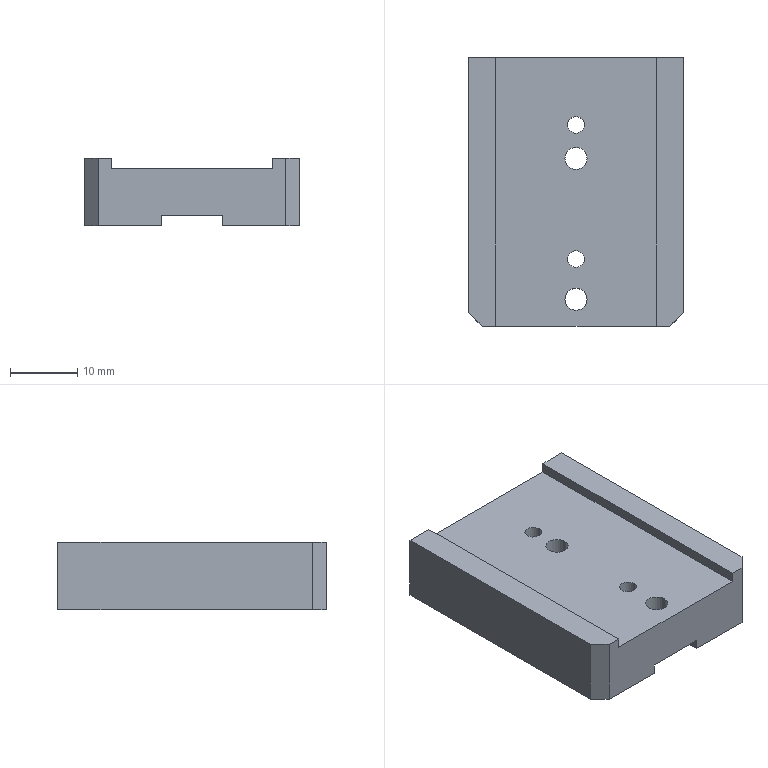Part | STEP file | 11-FG-E00911 | 1 solid | 32 faces | box 32 x 40 x 10 mm | volume 10413 mm3 | plane 16 | cylinder 12 | cone 4 | commonest cylinder face diameters 3.3 x8 2.5 x4
STEP:
#1=CARTESIAN_POINT('',(-24.467,23.184,2.85));
#2=VERTEX_POINT('',#1);
#3=CARTESIAN_POINT('',(-24.467,23.184,6.15));
#4=VERTEX_POINT('',#3);
#5=CARTESIAN_POINT('',(-24.467,23.184,4.5));
#6=DIRECTION('',(0.,1.,0.));
#7=DIRECTION('',(0.,0.,1.));
#8=AXIS2_PLACEMENT_3D('',#5,#6,#7);
#9=CIRCLE('',#8,1.65);
#10=EDGE_CURVE('',#2,#4,#9,.T.);
#11=ORIENTED_EDGE('',*,*,#10,.F.);
#12=CARTESIAN_POINT('',(-24.467,33.284,2.85));
#13=VERTEX_POINT('',#12);
#14=CARTESIAN_POINT('',(-24.467,33.284,2.85));
#15=DIRECTION('',(0.,1.,0.));
#16=VECTOR('',#15,1000.);
#17=LINE('',#14,#16);
#18=EDGE_CURVE('',#2,#13,#17,.T.);
#19=ORIENTED_EDGE('',*,*,#18,.T.);
#20=CARTESIAN_POINT('',(-24.467,33.284,6.15));
#21=VERTEX_POINT('',#20);
#22=CARTESIAN_POINT('',(-24.467,33.284,4.5));
#23=DIRECTION('',(0.,1.,0.));
#24=DIRECTION('',(0.,0.,1.));
#25=AXIS2_PLACEMENT_3D('',#22,#23,#24);
#26=CIRCLE('',#25,1.65);
#27=EDGE_CURVE('',#13,#21,#26,.T.);
#28=ORIENTED_EDGE('',*,*,#27,.T.);
#29=CARTESIAN_POINT('',(-24.467,33.284,6.15));
#30=DIRECTION('',(0.,1.,0.));
#31=VECTOR('',#30,1000.);
#32=LINE('',#29,#31);
#33=EDGE_CURVE('',#4,#21,#32,.T.);
#34=ORIENTED_EDGE('',*,*,#33,.F.);
#35=EDGE_LOOP('',(#11,#19,#28,#34));
#36=FACE_OUTER_BOUND('',#35,.T.);
#37=CARTESIAN_POINT('',(-24.467,33.284,4.5));
#38=DIRECTION('',(0.,1.,0.));
#39=DIRECTION('',(0.,0.,1.));
#40=AXIS2_PLACEMENT_3D('',#37,#38,#39);
#41=CYLINDRICAL_SURFACE('',#40,1.65);
#42=ADVANCED_FACE('',(#36),#41,.F.);
#43=CARTESIAN_POINT('',(-24.467,22.193,4.5));
#44=VERTEX_POINT('',#43);
#45=CARTESIAN_POINT('',(-24.467,23.184,6.15));
#46=DIRECTION('',(0.,0.515,0.8572));
#47=VECTOR('',#46,1000.);
#48=LINE('',#45,#47);
#49=EDGE_CURVE('',#44,#4,#48,.T.);
#50=ORIENTED_EDGE('',*,*,#49,.F.);
#51=CARTESIAN_POINT('',(-24.467,23.184,2.85));
#52=DIRECTION('',(0.,0.515,-0.8572));
#53=VECTOR('',#52,1000.);
#54=LINE('',#51,#53);
#55=EDGE_CURVE('',#44,#2,#54,.T.);
#56=ORIENTED_EDGE('',*,*,#55,.T.);
#57=ORIENTED_EDGE('',*,*,#10,.T.);
#58=EDGE_LOOP('',(#50,#56,#57));
#59=FACE_OUTER_BOUND('',#58,.T.);
#60=CARTESIAN_POINT('',(-24.467,23.184,4.5));
#61=DIRECTION('',(0.,1.,0.));
#62=DIRECTION('',(0.,0.,1.));
#63=AXIS2_PLACEMENT_3D('',#60,#61,#62);
#64=CONICAL_SURFACE('',#63,1.65,1.03);
#65=ADVANCED_FACE('',(#59),#64,.F.);
#66=CARTESIAN_POINT('',(-9.467,23.184,2.85));
#67=VERTEX_POINT('',#66);
#68=CARTESIAN_POINT('',(-9.467,23.184,6.15));
#69=VERTEX_POINT('',#68);
#70=CARTESIAN_POINT('',(-9.467,23.184,4.5));
#71=DIRECTION('',(0.,1.,0.));
#72=DIRECTION('',(0.,0.,1.));
#73=AXIS2_PLACEMENT_3D('',#70,#71,#72);
#74=CIRCLE('',#73,1.65);
#75=EDGE_CURVE('',#67,#69,#74,.T.);
#76=ORIENTED_EDGE('',*,*,#75,.F.);
#77=CARTESIAN_POINT('',(-9.467,33.284,2.85));
#78=VERTEX_POINT('',#77);
#79=CARTESIAN_POINT('',(-9.467,33.284,2.85));
#80=DIRECTION('',(0.,1.,0.));
#81=VECTOR('',#80,1000.);
#82=LINE('',#79,#81);
#83=EDGE_CURVE('',#67,#78,#82,.T.);
#84=ORIENTED_EDGE('',*,*,#83,.T.);
#85=CARTESIAN_POINT('',(-9.467,33.284,6.15));
#86=VERTEX_POINT('',#85);
#87=CARTESIAN_POINT('',(-9.467,33.284,4.5));
#88=DIRECTION('',(0.,1.,0.));
#89=DIRECTION('',(0.,0.,1.));
#90=AXIS2_PLACEMENT_3D('',#87,#88,#89);
#91=CIRCLE('',#90,1.65);
#92=EDGE_CURVE('',#78,#86,#91,.T.);
#93=ORIENTED_EDGE('',*,*,#92,.T.);
#94=CARTESIAN_POINT('',(-9.467,33.284,6.15));
#95=DIRECTION('',(0.,1.,0.));
#96=VECTOR('',#95,1000.);
#97=LINE('',#94,#96);
#98=EDGE_CURVE('',#69,#86,#97,.T.);
#99=ORIENTED_EDGE('',*,*,#98,.F.);
#100=EDGE_LOOP('',(#76,#84,#93,#99));
#101=FACE_OUTER_BOUND('',#100,.T.);
#102=CARTESIAN_POINT('',(-9.467,33.284,4.5));
#103=DIRECTION('',(0.,1.,0.));
#104=DIRECTION('',(0.,0.,1.));
#105=AXIS2_PLACEMENT_3D('',#102,#103,#104);
#106=CYLINDRICAL_SURFACE('',#105,1.65);
#107=ADVANCED_FACE('',(#101),#106,.F.);
#108=CARTESIAN_POINT('',(-9.467,22.193,4.5));
#109=VERTEX_POINT('',#108);
#110=CARTESIAN_POINT('',(-9.467,23.184,6.15));
#111=DIRECTION('',(0.,0.515,0.8572));
#112=VECTOR('',#111,1000.);
#113=LINE('',#110,#112);
#114=EDGE_CURVE('',#109,#69,#113,.T.);
#115=ORIENTED_EDGE('',*,*,#114,.F.);
#116=CARTESIAN_POINT('',(-9.467,23.184,2.85));
#117=DIRECTION('',(0.,0.515,-0.8572));
#118=VECTOR('',#117,1000.);
#119=LINE('',#116,#118);
#120=EDGE_CURVE('',#109,#67,#119,.T.);
#121=ORIENTED_EDGE('',*,*,#120,.T.);
#122=ORIENTED_EDGE('',*,*,#75,.T.);
#123=EDGE_LOOP('',(#115,#121,#122));
#124=FACE_OUTER_BOUND('',#123,.T.);
#125=CARTESIAN_POINT('',(-9.467,23.184,4.5));
#126=DIRECTION('',(0.,1.,0.));
#127=DIRECTION('',(0.,0.,1.));
#128=AXIS2_PLACEMENT_3D('',#125,#126,#127);
#129=CONICAL_SURFACE('',#128,1.65,1.03);
#130=ADVANCED_FACE('',(#124),#129,.F.);
#131=CARTESIAN_POINT('',(-18.617,-2.716,1.5));
#132=VERTEX_POINT('',#131);
#133=CARTESIAN_POINT('',(-15.317,-2.716,1.5));
#134=VERTEX_POINT('',#133);
#135=CARTESIAN_POINT('',(-16.967,-2.716,1.5));
#136=DIRECTION('',(0.,0.,1.));
#137=DIRECTION('',(1.,0.,0.));
#138=AXIS2_PLACEMENT_3D('',#135,#136,#137);
#139=CIRCLE('',#138,1.65);
#140=EDGE_CURVE('',#132,#134,#139,.T.);
#141=ORIENTED_EDGE('',*,*,#140,.F.);
#142=CARTESIAN_POINT('',(-18.617,-2.716,8.5));
#143=VERTEX_POINT('',#142);
#144=CARTESIAN_POINT('',(-18.617,-2.716,8.5));
#145=DIRECTION('',(0.,0.,1.));
#146=VECTOR('',#145,1000.);
#147=LINE('',#144,#146);
#148=EDGE_CURVE('',#132,#143,#147,.T.);
#149=ORIENTED_EDGE('',*,*,#148,.T.);
#150=CARTESIAN_POINT('',(-15.317,-2.716,8.5));
#151=VERTEX_POINT('',#150);
#152=CARTESIAN_POINT('',(-16.967,-2.716,8.5));
#153=DIRECTION('',(0.,0.,1.));
#154=DIRECTION('',(1.,0.,0.));
#155=AXIS2_PLACEMENT_3D('',#152,#153,#154);
#156=CIRCLE('',#155,1.65);
#157=EDGE_CURVE('',#143,#151,#156,.T.);
#158=ORIENTED_EDGE('',*,*,#157,.T.);
#159=CARTESIAN_POINT('',(-15.317,-2.716,8.5));
#160=DIRECTION('',(0.,0.,1.));
#161=VECTOR('',#160,1000.);
#162=LINE('',#159,#161);
#163=EDGE_CURVE('',#134,#151,#162,.T.);
#164=ORIENTED_EDGE('',*,*,#163,.F.);
#165=EDGE_LOOP('',(#141,#149,#158,#164));
#166=FACE_OUTER_BOUND('',#165,.T.);
#167=CARTESIAN_POINT('',(-16.967,-2.716,8.5));
#168=DIRECTION('',(0.,0.,1.));
#169=DIRECTION('',(1.,0.,0.));
#170=AXIS2_PLACEMENT_3D('',#167,#168,#169);
#171=CYLINDRICAL_SURFACE('',#170,1.65);
#172=ADVANCED_FACE('',(#166),#171,.F.);
#173=CARTESIAN_POINT('',(-18.617,18.284,1.5));
#174=VERTEX_POINT('',#173);
#175=CARTESIAN_POINT('',(-15.317,18.284,1.5));
#176=VERTEX_POINT('',#175);
#177=CARTESIAN_POINT('',(-16.967,18.284,1.5));
#178=DIRECTION('',(0.,0.,1.));
#179=DIRECTION('',(1.,0.,0.));
#180=AXIS2_PLACEMENT_3D('',#177,#178,#179);
#181=CIRCLE('',#180,1.65);
#182=EDGE_CURVE('',#174,#176,#181,.T.);
#183=ORIENTED_EDGE('',*,*,#182,.F.);
#184=CARTESIAN_POINT('',(-18.617,18.284,8.5));
#185=VERTEX_POINT('',#184);
#186=CARTESIAN_POINT('',(-18.617,18.284,8.5));
#187=DIRECTION('',(0.,0.,1.));
#188=VECTOR('',#187,1000.);
#189=LINE('',#186,#188);
#190=EDGE_CURVE('',#174,#185,#189,.T.);
#191=ORIENTED_EDGE('',*,*,#190,.T.);
#192=CARTESIAN_POINT('',(-15.317,18.284,8.5));
#193=VERTEX_POINT('',#192);
#194=CARTESIAN_POINT('',(-16.967,18.284,8.5));
#195=DIRECTION('',(0.,0.,1.));
#196=DIRECTION('',(1.,0.,0.));
#197=AXIS2_PLACEMENT_3D('',#194,#195,#196);
#198=CIRCLE('',#197,1.65);
#199=EDGE_CURVE('',#185,#193,#198,.T.);
#200=ORIENTED_EDGE('',*,*,#199,.T.);
#201=CARTESIAN_POINT('',(-15.317,18.284,8.5));
#202=DIRECTION('',(0.,0.,1.));
#203=VECTOR('',#202,1000.);
#204=LINE('',#201,#203);
#205=EDGE_CURVE('',#176,#193,#204,.T.);
#206=ORIENTED_EDGE('',*,*,#205,.F.);
#207=EDGE_LOOP('',(#183,#191,#200,#206));
#208=FACE_OUTER_BOUND('',#207,.T.);
#209=CARTESIAN_POINT('',(-16.967,18.284,8.5));
#210=DIRECTION('',(0.,0.,1.));
#211=DIRECTION('',(1.,0.,0.));
#212=AXIS2_PLACEMENT_3D('',#209,#210,#211);
#213=CYLINDRICAL_SURFACE('',#212,1.65);
#214=ADVANCED_FACE('',(#208),#213,.F.);
#215=CARTESIAN_POINT('',(-18.217,3.284,8.5));
#216=VERTEX_POINT('',#215);
#217=CARTESIAN_POINT('',(-15.717,3.284,8.5));
#218=VERTEX_POINT('',#217);
#219=CARTESIAN_POINT('',(-16.967,3.284,8.5));
#220=DIRECTION('',(0.,0.,1.));
#221=DIRECTION('',(1.,0.,0.));
#222=AXIS2_PLACEMENT_3D('',#219,#220,#221);
#223=CIRCLE('',#222,1.25);
#224=EDGE_CURVE('',#216,#218,#223,.T.);
#225=ORIENTED_EDGE('',*,*,#224,.T.);
#226=CARTESIAN_POINT('',(-15.717,3.284,1.5));
#227=VERTEX_POINT('',#226);
#228=CARTESIAN_POINT('',(-15.717,3.284,1.5));
#229=DIRECTION('',(0.,0.,-1.));
#230=VECTOR('',#229,1000.);
#231=LINE('',#228,#230);
#232=EDGE_CURVE('',#218,#227,#231,.T.);
#233=ORIENTED_EDGE('',*,*,#232,.T.);
#234=CARTESIAN_POINT('',(-18.217,3.284,1.5));
#235=VERTEX_POINT('',#234);
#236=CARTESIAN_POINT('',(-16.967,3.284,1.5));
#237=DIRECTION('',(0.,0.,-1.));
#238=DIRECTION('',(-1.,0.,0.));
#239=AXIS2_PLACEMENT_3D('',#236,#237,#238);
#240=CIRCLE('',#239,1.25);
#241=EDGE_CURVE('',#227,#235,#240,.T.);
#242=ORIENTED_EDGE('',*,*,#241,.T.);
#243=CARTESIAN_POINT('',(-18.217,3.284,1.5));
#244=DIRECTION('',(0.,0.,-1.));
#245=VECTOR('',#244,1000.);
#246=LINE('',#243,#245);
#247=EDGE_CURVE('',#216,#235,#246,.T.);
#248=ORIENTED_EDGE('',*,*,#247,.F.);
#249=EDGE_LOOP('',(#225,#233,#242,#248));
#250=FACE_OUTER_BOUND('',#249,.T.);
#251=CARTESIAN_POINT('',(-16.967,3.284,1.5));
#252=DIRECTION('',(0.,0.,-1.));
#253=DIRECTION('',(-1.,0.,0.));
#254=AXIS2_PLACEMENT_3D('',#251,#252,#253);
#255=CYLINDRICAL_SURFACE('',#254,1.25);
#256=ADVANCED_FACE('',(#250),#255,.F.);
#257=CARTESIAN_POINT('',(-18.217,23.284,8.5));
#258=VERTEX_POINT('',#257);
#259=CARTESIAN_POINT('',(-15.717,23.284,8.5));
#260=VERTEX_POINT('',#259);
#261=CARTESIAN_POINT('',(-16.967,23.284,8.5));
#262=DIRECTION('',(0.,0.,1.));
#263=DIRECTION('',(1.,0.,0.));
#264=AXIS2_PLACEMENT_3D('',#261,#262,#263);
#265=CIRCLE('',#264,1.25);
#266=EDGE_CURVE('',#258,#260,#265,.T.);
#267=ORIENTED_EDGE('',*,*,#266,.T.);
#268=CARTESIAN_POINT('',(-15.717,23.284,1.5));
#269=VERTEX_POINT('',#268);
#270=CARTESIAN_POINT('',(-15.717,23.284,1.5));
#271=DIRECTION('',(0.,0.,-1.));
#272=VECTOR('',#271,1000.);
#273=LINE('',#270,#272);
#274=EDGE_CURVE('',#260,#269,#273,.T.);
#275=ORIENTED_EDGE('',*,*,#274,.T.);
#276=CARTESIAN_POINT('',(-18.217,23.284,1.5));
#277=VERTEX_POINT('',#276);
#278=CARTESIAN_POINT('',(-16.967,23.284,1.5));
#279=DIRECTION('',(0.,0.,-1.));
#280=DIRECTION('',(-1.,0.,0.));
#281=AXIS2_PLACEMENT_3D('',#278,#279,#280);
#282=CIRCLE('',#281,1.25);
#283=EDGE_CURVE('',#269,#277,#282,.T.);
#284=ORIENTED_EDGE('',*,*,#283,.T.);
#285=CARTESIAN_POINT('',(-18.217,23.284,1.5));
#286=DIRECTION('',(0.,0.,-1.));
#287=VECTOR('',#286,1000.);
#288=LINE('',#285,#287);
#289=EDGE_CURVE('',#258,#277,#288,.T.);
#290=ORIENTED_EDGE('',*,*,#289,.F.);
#291=EDGE_LOOP('',(#267,#275,#284,#290));
#292=FACE_OUTER_BOUND('',#291,.T.);
#293=CARTESIAN_POINT('',(-16.967,23.284,1.5));
#294=DIRECTION('',(0.,0.,-1.));
#295=DIRECTION('',(-1.,0.,0.));
#296=AXIS2_PLACEMENT_3D('',#293,#294,#295);
#297=CYLINDRICAL_SURFACE('',#296,1.25);
#298=ADVANCED_FACE('',(#292),#297,.F.);
#299=CARTESIAN_POINT('',(-12.467,-6.716,0.));
#300=VERTEX_POINT('',#299);
#301=CARTESIAN_POINT('',(-2.967,-6.716,0.));
#302=VERTEX_POINT('',#301);
#303=CARTESIAN_POINT('',(-32.967,-6.716,0.));
#304=DIRECTION('',(1.,0.,0.));
#305=VECTOR('',#304,1000.);
#306=LINE('',#303,#305);
#307=EDGE_CURVE('',#300,#302,#306,.T.);
#308=ORIENTED_EDGE('',*,*,#307,.F.);
#309=CARTESIAN_POINT('',(-12.467,33.284,0.));
#310=VERTEX_POINT('',#309);
#311=CARTESIAN_POINT('',(-12.467,-6.716,0.));
#312=DIRECTION('',(0.,1.,0.));
#313=VECTOR('',#312,1000.);
#314=LINE('',#311,#313);
#315=EDGE_CURVE('',#300,#310,#314,.T.);
#316=ORIENTED_EDGE('',*,*,#315,.T.);
#317=CARTESIAN_POINT('',(-0.9669,33.284,0.));
#318=VERTEX_POINT('',#317);
#319=CARTESIAN_POINT('',(-32.967,33.284,0.));
#320=DIRECTION('',(-1.,0.,0.));
#321=VECTOR('',#320,1000.);
#322=LINE('',#319,#321);
#323=EDGE_CURVE('',#318,#310,#322,.T.);
#324=ORIENTED_EDGE('',*,*,#323,.F.);
#325=CARTESIAN_POINT('',(-0.9669,-4.716,0.));
#326=VERTEX_POINT('',#325);
#327=CARTESIAN_POINT('',(-0.9669,33.284,0.));
#328=DIRECTION('',(0.,1.,0.));
#329=VECTOR('',#328,1000.);
#330=LINE('',#327,#329);
#331=EDGE_CURVE('',#326,#318,#330,.T.);
#332=ORIENTED_EDGE('',*,*,#331,.F.);
#333=CARTESIAN_POINT('',(-0.9669,-4.716,0.));
#334=DIRECTION('',(-0.7071,-0.7071,0.));
#335=VECTOR('',#334,1000.);
#336=LINE('',#333,#335);
#337=EDGE_CURVE('',#326,#302,#336,.T.);
#338=ORIENTED_EDGE('',*,*,#337,.T.);
#339=EDGE_LOOP('',(#308,#316,#324,#332,#338));
#340=FACE_OUTER_BOUND('',#339,.T.);
#341=CARTESIAN_POINT('',(-32.967,-6.716,0.));
#342=DIRECTION('',(0.,0.,1.));
#343=DIRECTION('',(1.,0.,0.));
#344=AXIS2_PLACEMENT_3D('',#341,#342,#343);
#345=PLANE('',#344);
#346=ADVANCED_FACE('',(#340),#345,.F.);
#347=CARTESIAN_POINT('',(-24.467,33.284,4.5));
#348=DIRECTION('',(0.,1.,0.));
#349=DIRECTION('',(0.,0.,1.));
#350=AXIS2_PLACEMENT_3D('',#347,#348,#349);
#351=CIRCLE('',#350,1.65);
#352=EDGE_CURVE('',#21,#13,#351,.T.);
#353=ORIENTED_EDGE('',*,*,#352,.F.);
#354=ORIENTED_EDGE('',*,*,#27,.F.);
#355=EDGE_LOOP('',(#353,#354));
#356=FACE_BOUND('',#355,.T.);
#357=CARTESIAN_POINT('',(-9.467,33.284,4.5));
#358=DIRECTION('',(0.,1.,0.));
#359=DIRECTION('',(0.,0.,1.));
#360=AXIS2_PLACEMENT_3D('',#357,#358,#359);
#361=CIRCLE('',#360,1.65);
#362=EDGE_CURVE('',#86,#78,#361,.T.);
#363=ORIENTED_EDGE('',*,*,#362,.F.);
#364=ORIENTED_EDGE('',*,*,#92,.F.);
#365=EDGE_LOOP('',(#363,#364));
#366=FACE_BOUND('',#365,.T.);
#367=ORIENTED_EDGE('',*,*,#323,.T.);
#368=CARTESIAN_POINT('',(-12.467,33.284,1.5));
#369=VERTEX_POINT('',#368);
#370=CARTESIAN_POINT('',(-12.467,33.284,10.));
#371=DIRECTION('',(0.,0.,1.));
#372=VECTOR('',#371,1000.);
#373=LINE('',#370,#372);
#374=EDGE_CURVE('',#310,#369,#373,.T.);
#375=ORIENTED_EDGE('',*,*,#374,.T.);
#376=CARTESIAN_POINT('',(-21.467,33.284,1.5));
#377=VERTEX_POINT('',#376);
#378=CARTESIAN_POINT('',(-32.967,33.284,1.5));
#379=DIRECTION('',(-1.,0.,0.));
#380=VECTOR('',#379,1000.);
#381=LINE('',#378,#380);
#382=EDGE_CURVE('',#369,#377,#381,.T.);
#383=ORIENTED_EDGE('',*,*,#382,.T.);
#384=CARTESIAN_POINT('',(-21.467,33.284,0.));
#385=VERTEX_POINT('',#384);
#386=CARTESIAN_POINT('',(-21.467,33.284,10.));
#387=DIRECTION('',(0.,0.,-1.));
#388=VECTOR('',#387,1000.);
#389=LINE('',#386,#388);
#390=EDGE_CURVE('',#377,#385,#389,.T.);
#391=ORIENTED_EDGE('',*,*,#390,.T.);
#392=CARTESIAN_POINT('',(-32.967,33.284,0.));
#393=VERTEX_POINT('',#392);
#394=CARTESIAN_POINT('',(-32.967,33.284,0.));
#395=DIRECTION('',(-1.,0.,0.));
#396=VECTOR('',#395,1000.);
#397=LINE('',#394,#396);
#398=EDGE_CURVE('',#385,#393,#397,.T.);
#399=ORIENTED_EDGE('',*,*,#398,.T.);
#400=CARTESIAN_POINT('',(-32.967,33.284,10.));
#401=VERTEX_POINT('',#400);
#402=CARTESIAN_POINT('',(-32.967,33.284,10.));
#403=DIRECTION('',(0.,0.,-1.));
#404=VECTOR('',#403,1000.);
#405=LINE('',#402,#404);
#406=EDGE_CURVE('',#401,#393,#405,.T.);
#407=ORIENTED_EDGE('',*,*,#406,.F.);
#408=CARTESIAN_POINT('',(-28.967,33.284,10.));
#409=VERTEX_POINT('',#408);
#410=CARTESIAN_POINT('',(-32.967,33.284,10.));
#411=DIRECTION('',(-1.,0.,0.));
#412=VECTOR('',#411,1000.);
#413=LINE('',#410,#412);
#414=EDGE_CURVE('',#409,#401,#413,.T.);
#415=ORIENTED_EDGE('',*,*,#414,.F.);
#416=CARTESIAN_POINT('',(-28.967,33.284,8.5));
#417=VERTEX_POINT('',#416);
#418=CARTESIAN_POINT('',(-28.967,33.284,8.5));
#419=DIRECTION('',(0.,0.,1.));
#420=VECTOR('',#419,1000.);
#421=LINE('',#418,#420);
#422=EDGE_CURVE('',#417,#409,#421,.T.);
#423=ORIENTED_EDGE('',*,*,#422,.F.);
#424=CARTESIAN_POINT('',(-4.967,33.284,8.5));
#425=VERTEX_POINT('',#424);
#426=CARTESIAN_POINT('',(-28.967,33.284,8.5));
#427=DIRECTION('',(-1.,0.,0.));
#428=VECTOR('',#427,1000.);
#429=LINE('',#426,#428);
#430=EDGE_CURVE('',#425,#417,#429,.T.);
#431=ORIENTED_EDGE('',*,*,#430,.F.);
#432=CARTESIAN_POINT('',(-4.967,33.284,10.));
#433=VERTEX_POINT('',#432);
#434=CARTESIAN_POINT('',(-4.967,33.284,8.5));
#435=DIRECTION('',(0.,0.,1.));
#436=VECTOR('',#435,1000.);
#437=LINE('',#434,#436);
#438=EDGE_CURVE('',#425,#433,#437,.T.);
#439=ORIENTED_EDGE('',*,*,#438,.T.);
#440=CARTESIAN_POINT('',(-0.9669,33.284,10.));
#441=VERTEX_POINT('',#440);
#442=CARTESIAN_POINT('',(-32.967,33.284,10.));
#443=DIRECTION('',(-1.,0.,0.));
#444=VECTOR('',#443,1000.);
#445=LINE('',#442,#444);
#446=EDGE_CURVE('',#441,#433,#445,.T.);
#447=ORIENTED_EDGE('',*,*,#446,.F.);
#448=CARTESIAN_POINT('',(-0.9669,33.284,10.));
#449=DIRECTION('',(0.,0.,-1.));
#450=VECTOR('',#449,1000.);
#451=LINE('',#448,#450);
#452=EDGE_CURVE('',#441,#318,#451,.T.);
#453=ORIENTED_EDGE('',*,*,#452,.T.);
#454=EDGE_LOOP('',(#367,#375,#383,#391,#399,#407,#415,#423,#431,#439,#447,#453));
#455=FACE_OUTER_BOUND('',#454,.T.);
#456=CARTESIAN_POINT('',(-32.967,33.284,10.));
#457=DIRECTION('',(0.,-1.,0.));
#458=DIRECTION('',(0.,0.,-1.));
#459=AXIS2_PLACEMENT_3D('',#456,#457,#458);
#460=PLANE('',#459);
#461=ADVANCED_FACE('',(#356,#366,#455),#460,.F.);
#462=CARTESIAN_POINT('',(-32.967,-4.716,10.));
#463=VERTEX_POINT('',#462);
#464=CARTESIAN_POINT('',(-32.967,33.284,10.));
#465=DIRECTION('',(0.,-1.,0.));
#466=VECTOR('',#465,1000.);
#467=LINE('',#464,#466);
#468=EDGE_CURVE('',#401,#463,#467,.T.);
#469=ORIENTED_EDGE('',*,*,#468,.T.);
#470=CARTESIAN_POINT('',(-30.967,-6.716,10.));
#471=VERTEX_POINT('',#470);
#472=CARTESIAN_POINT('',(-31.967,-5.716,10.));
#473=DIRECTION('',(0.7071,-0.7071,0.));
#474=VECTOR('',#473,1000.);
#475=LINE('',#472,#474);
#476=EDGE_CURVE('',#463,#471,#475,.T.);
#477=ORIENTED_EDGE('',*,*,#476,.T.);
#478=CARTESIAN_POINT('',(-28.967,-6.716,10.));
#479=VERTEX_POINT('',#478);
#480=CARTESIAN_POINT('',(-32.967,-6.716,10.));
#481=DIRECTION('',(1.,0.,0.));
#482=VECTOR('',#481,1000.);
#483=LINE('',#480,#482);
#484=EDGE_CURVE('',#471,#479,#483,.T.);
#485=ORIENTED_EDGE('',*,*,#484,.T.);
#486=CARTESIAN_POINT('',(-28.967,33.284,10.));
#487=DIRECTION('',(0.,-1.,0.));
#488=VECTOR('',#487,1000.);
#489=LINE('',#486,#488);
#490=EDGE_CURVE('',#409,#479,#489,.T.);
#491=ORIENTED_EDGE('',*,*,#490,.F.);
#492=ORIENTED_EDGE('',*,*,#414,.T.);
#493=EDGE_LOOP('',(#469,#477,#485,#491,#492));
#494=FACE_OUTER_BOUND('',#493,.T.);
#495=CARTESIAN_POINT('',(-32.967,-6.716,10.));
#496=DIRECTION('',(0.,0.,1.));
#497=DIRECTION('',(1.,0.,0.));
#498=AXIS2_PLACEMENT_3D('',#495,#496,#497);
#499=PLANE('',#498);
#500=ADVANCED_FACE('',(#494),#499,.T.);
#501=CARTESIAN_POINT('',(-32.967,-4.716,0.));
#502=VERTEX_POINT('',#501);
#503=CARTESIAN_POINT('',(-32.967,33.284,0.));
#504=DIRECTION('',(0.,-1.,0.));
#505=VECTOR('',#504,1000.);
#506=LINE('',#503,#505);
#507=EDGE_CURVE('',#393,#502,#506,.T.);
#508=ORIENTED_EDGE('',*,*,#507,.T.);
#509=CARTESIAN_POINT('',(-32.967,-4.716,10.));
#510=DIRECTION('',(0.,0.,1.));
#511=VECTOR('',#510,1000.);
#512=LINE('',#509,#511);
#513=EDGE_CURVE('',#502,#463,#512,.T.);
#514=ORIENTED_EDGE('',*,*,#513,.T.);
#515=ORIENTED_EDGE('',*,*,#468,.F.);
#516=ORIENTED_EDGE('',*,*,#406,.T.);
#517=EDGE_LOOP('',(#508,#514,#515,#516));
#518=FACE_OUTER_BOUND('',#517,.T.);
#519=CARTESIAN_POINT('',(-32.967,33.284,10.));
#520=DIRECTION('',(1.,0.,0.));
#521=DIRECTION('',(0.,1.,0.));
#522=AXIS2_PLACEMENT_3D('',#519,#520,#521);
#523=PLANE('',#522);
#524=ADVANCED_FACE('',(#518),#523,.F.);
#525=CARTESIAN_POINT('',(-12.467,-6.716,1.5));
#526=VERTEX_POINT('',#525);
#527=CARTESIAN_POINT('',(-21.467,-6.716,1.5));
#528=VERTEX_POINT('',#527);
#529=CARTESIAN_POINT('',(-12.467,-6.716,1.5));
#530=DIRECTION('',(-1.,0.,0.));
#531=VECTOR('',#530,1000.);
#532=LINE('',#529,#531);
#533=EDGE_CURVE('',#526,#528,#532,.T.);
#534=ORIENTED_EDGE('',*,*,#533,.F.);
#535=CARTESIAN_POINT('',(-12.467,-6.716,0.));
#536=DIRECTION('',(0.,0.,1.));
#537=VECTOR('',#536,1000.);
#538=LINE('',#535,#537);
#539=EDGE_CURVE('',#300,#526,#538,.T.);
#540=ORIENTED_EDGE('',*,*,#539,.F.);
#541=ORIENTED_EDGE('',*,*,#307,.T.);
#542=CARTESIAN_POINT('',(-2.967,-6.716,10.));
#543=VERTEX_POINT('',#542);
#544=CARTESIAN_POINT('',(-2.967,-6.716,10.));
#545=DIRECTION('',(0.,0.,1.));
#546=VECTOR('',#545,1000.);
#547=LINE('',#544,#546);
#548=EDGE_CURVE('',#302,#543,#547,.T.);
#549=ORIENTED_EDGE('',*,*,#548,.T.);
#550=CARTESIAN_POINT('',(-4.967,-6.716,10.));
#551=VERTEX_POINT('',#550);
#552=CARTESIAN_POINT('',(-32.967,-6.716,10.));
#553=DIRECTION('',(1.,0.,0.));
#554=VECTOR('',#553,1000.);
#555=LINE('',#552,#554);
#556=EDGE_CURVE('',#551,#543,#555,.T.);
#557=ORIENTED_EDGE('',*,*,#556,.F.);
#558=CARTESIAN_POINT('',(-4.967,-6.716,8.5));
#559=VERTEX_POINT('',#558);
#560=CARTESIAN_POINT('',(-4.967,-6.716,8.5));
#561=DIRECTION('',(0.,0.,1.));
#562=VECTOR('',#561,1000.);
#563=LINE('',#560,#562);
#564=EDGE_CURVE('',#559,#551,#563,.T.);
#565=ORIENTED_EDGE('',*,*,#564,.F.);
#566=CARTESIAN_POINT('',(-28.967,-6.716,8.5));
#567=VERTEX_POINT('',#566);
#568=CARTESIAN_POINT('',(-28.967,-6.716,8.5));
#569=DIRECTION('',(1.,0.,0.));
#570=VECTOR('',#569,1000.);
#571=LINE('',#568,#570);
#572=EDGE_CURVE('',#567,#559,#571,.T.);
#573=ORIENTED_EDGE('',*,*,#572,.F.);
#574=CARTESIAN_POINT('',(-28.967,-6.716,8.5));
#575=DIRECTION('',(0.,0.,1.));
#576=VECTOR('',#575,1000.);
#577=LINE('',#574,#576);
#578=EDGE_CURVE('',#567,#479,#577,.T.);
#579=ORIENTED_EDGE('',*,*,#578,.T.);
#580=ORIENTED_EDGE('',*,*,#484,.F.);
#581=CARTESIAN_POINT('',(-30.967,-6.716,0.));
#582=VERTEX_POINT('',#581);
#583=CARTESIAN_POINT('',(-30.967,-6.716,10.));
#584=DIRECTION('',(0.,0.,-1.));
#585=VECTOR('',#584,1000.);
#586=LINE('',#583,#585);
#587=EDGE_CURVE('',#471,#582,#586,.T.);
#588=ORIENTED_EDGE('',*,*,#587,.T.);
#589=CARTESIAN_POINT('',(-21.467,-6.716,0.));
#590=VERTEX_POINT('',#589);
#591=CARTESIAN_POINT('',(-32.967,-6.716,0.));
#592=DIRECTION('',(1.,0.,0.));
#593=VECTOR('',#592,1000.);
#594=LINE('',#591,#593);
#595=EDGE_CURVE('',#582,#590,#594,.T.);
#596=ORIENTED_EDGE('',*,*,#595,.T.);
#597=CARTESIAN_POINT('',(-21.467,-6.716,0.));
#598=DIRECTION('',(0.,0.,-1.));
#599=VECTOR('',#598,1000.);
#600=LINE('',#597,#599);
#601=EDGE_CURVE('',#528,#590,#600,.T.);
#602=ORIENTED_EDGE('',*,*,#601,.F.);
#603=EDGE_LOOP('',(#534,#540,#541,#549,#557,#565,#573,#579,#580,#588,#596,#602));
#604=FACE_OUTER_BOUND('',#603,.T.);
#605=CARTESIAN_POINT('',(-32.967,-6.716,10.));
#606=DIRECTION('',(0.,1.,0.));
#607=DIRECTION('',(0.,0.,1.));
#608=AXIS2_PLACEMENT_3D('',#605,#606,#607);
#609=PLANE('',#608);
#610=ADVANCED_FACE('',(#604),#609,.F.);
#611=CARTESIAN_POINT('',(-0.9669,-4.716,10.));
#612=VERTEX_POINT('',#611);
#613=CARTESIAN_POINT('',(-0.9669,33.284,10.));
#614=DIRECTION('',(0.,1.,0.));
#615=VECTOR('',#614,1000.);
#616=LINE('',#613,#615);
#617=EDGE_CURVE('',#612,#441,#616,.T.);
#618=ORIENTED_EDGE('',*,*,#617,.F.);
#619=CARTESIAN_POINT('',(-0.9669,-4.716,10.));
#620=DIRECTION('',(0.,0.,-1.));
#621=VECTOR('',#620,1000.);
#622=LINE('',#619,#621);
#623=EDGE_CURVE('',#612,#326,#622,.T.);
#624=ORIENTED_EDGE('',*,*,#623,.T.);
#625=ORIENTED_EDGE('',*,*,#331,.T.);
#626=ORIENTED_EDGE('',*,*,#452,.F.);
#627=EDGE_LOOP('',(#618,#624,#625,#626));
#628=FACE_OUTER_BOUND('',#627,.T.);
#629=CARTESIAN_POINT('',(-0.9669,33.284,10.));
#630=DIRECTION('',(-1.,0.,0.));
#631=DIRECTION('',(0.,-1.,0.));
#632=AXIS2_PLACEMENT_3D('',#629,#630,#631);
#633=PLANE('',#632);
#634=ADVANCED_FACE('',(#628),#633,.F.);
#635=ORIENTED_EDGE('',*,*,#556,.T.);
#636=CARTESIAN_POINT('',(-17.967,-21.716,10.));
#637=DIRECTION('',(0.7071,0.7071,0.));
#638=VECTOR('',#637,1000.);
#639=LINE('',#636,#638);
#640=EDGE_CURVE('',#543,#612,#639,.T.);
#641=ORIENTED_EDGE('',*,*,#640,.T.);
#642=ORIENTED_EDGE('',*,*,#617,.T.);
#643=ORIENTED_EDGE('',*,*,#446,.T.);
#644=CARTESIAN_POINT('',(-4.967,33.284,10.));
#645=DIRECTION('',(0.,1.,0.));
#646=VECTOR('',#645,1000.);
#647=LINE('',#644,#646);
#648=EDGE_CURVE('',#551,#433,#647,.T.);
#649=ORIENTED_EDGE('',*,*,#648,.F.);
#650=EDGE_LOOP('',(#635,#641,#642,#643,#649));
#651=FACE_OUTER_BOUND('',#650,.T.);
#652=CARTESIAN_POINT('',(-32.967,-6.716,10.));
#653=DIRECTION('',(0.,0.,1.));
#654=DIRECTION('',(1.,0.,0.));
#655=AXIS2_PLACEMENT_3D('',#652,#653,#654);
#656=PLANE('',#655);
#657=ADVANCED_FACE('',(#651),#656,.T.);
#658=ORIENTED_EDGE('',*,*,#398,.F.);
#659=CARTESIAN_POINT('',(-21.467,-6.716,0.));
#660=DIRECTION('',(0.,-1.,0.));
#661=VECTOR('',#660,1000.);
#662=LINE('',#659,#661);
#663=EDGE_CURVE('',#385,#590,#662,.T.);
#664=ORIENTED_EDGE('',*,*,#663,.T.);
#665=ORIENTED_EDGE('',*,*,#595,.F.);
#666=CARTESIAN_POINT('',(-30.967,-6.716,0.));
#667=DIRECTION('',(-0.7071,0.7071,0.));
#668=VECTOR('',#667,1000.);
#669=LINE('',#666,#668);
#670=EDGE_CURVE('',#582,#502,#669,.T.);
#671=ORIENTED_EDGE('',*,*,#670,.T.);
#672=ORIENTED_EDGE('',*,*,#507,.F.);
#673=EDGE_LOOP('',(#658,#664,#665,#671,#672));
#674=FACE_OUTER_BOUND('',#673,.T.);
#675=CARTESIAN_POINT('',(-32.967,-6.716,0.));
#676=DIRECTION('',(0.,0.,1.));
#677=DIRECTION('',(1.,0.,0.));
#678=AXIS2_PLACEMENT_3D('',#675,#676,#677);
#679=PLANE('',#678);
#680=ADVANCED_FACE('',(#674),#679,.F.);
#681=ORIENTED_EDGE('',*,*,#490,.T.);
#682=ORIENTED_EDGE('',*,*,#578,.F.);
#683=CARTESIAN_POINT('',(-28.967,33.284,8.5));
#684=DIRECTION('',(0.,-1.,0.));
#685=VECTOR('',#684,1000.);
#686=LINE('',#683,#685);
#687=EDGE_CURVE('',#417,#567,#686,.T.);
#688=ORIENTED_EDGE('',*,*,#687,.F.);
#689=ORIENTED_EDGE('',*,*,#422,.T.);
#690=EDGE_LOOP('',(#681,#682,#688,#689));
#691=FACE_OUTER_BOUND('',#690,.T.);
#692=CARTESIAN_POINT('',(-28.967,33.284,8.5));
#693=DIRECTION('',(-1.,0.,0.));
#694=DIRECTION('',(0.,-1.,0.));
#695=AXIS2_PLACEMENT_3D('',#692,#693,#694);
#696=PLANE('',#695);
#697=ADVANCED_FACE('',(#691),#696,.F.);
#698=ORIENTED_EDGE('',*,*,#648,.T.);
#699=ORIENTED_EDGE('',*,*,#438,.F.);
#700=CARTESIAN_POINT('',(-4.967,33.284,8.5));
#701=DIRECTION('',(0.,1.,0.));
#702=VECTOR('',#701,1000.);
#703=LINE('',#700,#702);
#704=EDGE_CURVE('',#559,#425,#703,.T.);
#705=ORIENTED_EDGE('',*,*,#704,.F.);
#706=ORIENTED_EDGE('',*,*,#564,.T.);
#707=EDGE_LOOP('',(#698,#699,#705,#706));
#708=FACE_OUTER_BOUND('',#707,.T.);
#709=CARTESIAN_POINT('',(-4.967,33.284,8.5));
#710=DIRECTION('',(1.,0.,0.));
#711=DIRECTION('',(0.,1.,0.));
#712=AXIS2_PLACEMENT_3D('',#709,#710,#711);
#713=PLANE('',#712);
#714=ADVANCED_FACE('',(#708),#713,.F.);
#715=CARTESIAN_POINT('',(-16.967,-2.716,8.5));
#716=DIRECTION('',(0.,0.,1.));
#717=DIRECTION('',(1.,0.,0.));
#718=AXIS2_PLACEMENT_3D('',#715,#716,#717);
#719=CIRCLE('',#718,1.65);
#720=EDGE_CURVE('',#151,#143,#719,.T.);
#721=ORIENTED_EDGE('',*,*,#720,.F.);
#722=ORIENTED_EDGE('',*,*,#157,.F.);
#723=EDGE_LOOP('',(#721,#722));
#724=FACE_BOUND('',#723,.T.);
#725=CARTESIAN_POINT('',(-16.967,18.284,8.5));
#726=DIRECTION('',(0.,0.,1.));
#727=DIRECTION('',(1.,0.,0.));
#728=AXIS2_PLACEMENT_3D('',#725,#726,#727);
#729=CIRCLE('',#728,1.65);
#730=EDGE_CURVE('',#193,#185,#729,.T.);
#731=ORIENTED_EDGE('',*,*,#730,.F.);
#732=ORIENTED_EDGE('',*,*,#199,.F.);
#733=EDGE_LOOP('',(#731,#732));
#734=FACE_BOUND('',#733,.T.);
#735=ORIENTED_EDGE('',*,*,#224,.F.);
#736=CARTESIAN_POINT('',(-16.967,3.284,8.5));
#737=DIRECTION('',(0.,0.,1.));
#738=DIRECTION('',(1.,0.,0.));
#739=AXIS2_PLACEMENT_3D('',#736,#737,#738);
#740=CIRCLE('',#739,1.25);
#741=EDGE_CURVE('',#218,#216,#740,.T.);
#742=ORIENTED_EDGE('',*,*,#741,.F.);
#743=EDGE_LOOP('',(#735,#742));
#744=FACE_BOUND('',#743,.T.);
#745=ORIENTED_EDGE('',*,*,#266,.F.);
#746=CARTESIAN_POINT('',(-16.967,23.284,8.5));
#747=DIRECTION('',(0.,0.,1.));
#748=DIRECTION('',(1.,0.,0.));
#749=AXIS2_PLACEMENT_3D('',#746,#747,#748);
#750=CIRCLE('',#749,1.25);
#751=EDGE_CURVE('',#260,#258,#750,.T.);
#752=ORIENTED_EDGE('',*,*,#751,.F.);
#753=EDGE_LOOP('',(#745,#752));
#754=FACE_BOUND('',#753,.T.);
#755=ORIENTED_EDGE('',*,*,#687,.T.);
#756=ORIENTED_EDGE('',*,*,#572,.T.);
#757=ORIENTED_EDGE('',*,*,#704,.T.);
#758=ORIENTED_EDGE('',*,*,#430,.T.);
#759=EDGE_LOOP('',(#755,#756,#757,#758));
#760=FACE_OUTER_BOUND('',#759,.T.);
#761=CARTESIAN_POINT('',(-28.967,-6.716,8.5));
#762=DIRECTION('',(0.,0.,1.));
#763=DIRECTION('',(1.,0.,0.));
#764=AXIS2_PLACEMENT_3D('',#761,#762,#763);
#765=PLANE('',#764);
#766=ADVANCED_FACE('',(#724,#734,#744,#754,#760),#765,.T.);
#767=ORIENTED_EDGE('',*,*,#640,.F.);
#768=ORIENTED_EDGE('',*,*,#548,.F.);
#769=ORIENTED_EDGE('',*,*,#337,.F.);
#770=ORIENTED_EDGE('',*,*,#623,.F.);
#771=EDGE_LOOP('',(#767,#768,#769,#770));
#772=FACE_OUTER_BOUND('',#771,.T.);
#773=CARTESIAN_POINT('',(-0.9669,-4.716,10.));
#774=DIRECTION('',(-0.7071,0.7071,0.));
#775=DIRECTION('',(0.,0.,-1.));
#776=AXIS2_PLACEMENT_3D('',#773,#774,#775);
#777=PLANE('',#776);
#778=ADVANCED_FACE('',(#772),#777,.F.);
#779=ORIENTED_EDGE('',*,*,#476,.F.);
#780=ORIENTED_EDGE('',*,*,#513,.F.);
#781=ORIENTED_EDGE('',*,*,#670,.F.);
#782=ORIENTED_EDGE('',*,*,#587,.F.);
#783=EDGE_LOOP('',(#779,#780,#781,#782));
#784=FACE_OUTER_BOUND('',#783,.T.);
#785=CARTESIAN_POINT('',(-30.967,-6.716,10.));
#786=DIRECTION('',(0.7071,0.7071,0.));
#787=DIRECTION('',(0.,0.,-1.));
#788=AXIS2_PLACEMENT_3D('',#785,#786,#787);
#789=PLANE('',#788);
#790=ADVANCED_FACE('',(#784),#789,.F.);
#791=CARTESIAN_POINT('',(-16.967,-2.716,1.5));
#792=DIRECTION('',(0.,0.,1.));
#793=DIRECTION('',(1.,0.,0.));
#794=AXIS2_PLACEMENT_3D('',#791,#792,#793);
#795=CIRCLE('',#794,1.65);
#796=EDGE_CURVE('',#134,#132,#795,.T.);
#797=ORIENTED_EDGE('',*,*,#796,.T.);
#798=ORIENTED_EDGE('',*,*,#140,.T.);
#799=EDGE_LOOP('',(#797,#798));
#800=FACE_BOUND('',#799,.T.);
#801=CARTESIAN_POINT('',(-16.967,18.284,1.5));
#802=DIRECTION('',(0.,0.,1.));
#803=DIRECTION('',(1.,0.,0.));
#804=AXIS2_PLACEMENT_3D('',#801,#802,#803);
#805=CIRCLE('',#804,1.65);
#806=EDGE_CURVE('',#176,#174,#805,.T.);
#807=ORIENTED_EDGE('',*,*,#806,.T.);
#808=ORIENTED_EDGE('',*,*,#182,.T.);
#809=EDGE_LOOP('',(#807,#808));
#810=FACE_BOUND('',#809,.T.);
#811=CARTESIAN_POINT('',(-16.967,3.284,1.5));
#812=DIRECTION('',(0.,0.,-1.));
#813=DIRECTION('',(-1.,0.,0.));
#814=AXIS2_PLACEMENT_3D('',#811,#812,#813);
#815=CIRCLE('',#814,1.25);
#816=EDGE_CURVE('',#235,#227,#815,.T.);
#817=ORIENTED_EDGE('',*,*,#816,.F.);
#818=ORIENTED_EDGE('',*,*,#241,.F.);
#819=EDGE_LOOP('',(#817,#818));
#820=FACE_BOUND('',#819,.T.);
#821=CARTESIAN_POINT('',(-16.967,23.284,1.5));
#822=DIRECTION('',(0.,0.,-1.));
#823=DIRECTION('',(-1.,0.,0.));
#824=AXIS2_PLACEMENT_3D('',#821,#822,#823);
#825=CIRCLE('',#824,1.25);
#826=EDGE_CURVE('',#277,#269,#825,.T.);
#827=ORIENTED_EDGE('',*,*,#826,.F.);
#828=ORIENTED_EDGE('',*,*,#283,.F.);
#829=EDGE_LOOP('',(#827,#828));
#830=FACE_BOUND('',#829,.T.);
#831=CARTESIAN_POINT('',(-12.467,144.284,1.5));
#832=DIRECTION('',(0.,-1.,0.));
#833=VECTOR('',#832,1000.);
#834=LINE('',#831,#833);
#835=EDGE_CURVE('',#369,#526,#834,.T.);
#836=ORIENTED_EDGE('',*,*,#835,.T.);
#837=ORIENTED_EDGE('',*,*,#533,.T.);
#838=CARTESIAN_POINT('',(-21.467,144.284,1.5));
#839=DIRECTION('',(0.,-1.,0.));
#840=VECTOR('',#839,1000.);
#841=LINE('',#838,#840);
#842=EDGE_CURVE('',#377,#528,#841,.T.);
#843=ORIENTED_EDGE('',*,*,#842,.F.);
#844=ORIENTED_EDGE('',*,*,#382,.F.);
#845=EDGE_LOOP('',(#836,#837,#843,#844));
#846=FACE_OUTER_BOUND('',#845,.T.);
#847=CARTESIAN_POINT('',(-12.467,144.284,1.5));
#848=DIRECTION('',(0.,0.,1.));
#849=DIRECTION('',(1.,0.,0.));
#850=AXIS2_PLACEMENT_3D('',#847,#848,#849);
#851=PLANE('',#850);
#852=ADVANCED_FACE('',(#800,#810,#820,#830,#846),#851,.F.);
#853=ORIENTED_EDGE('',*,*,#315,.F.);
#854=ORIENTED_EDGE('',*,*,#539,.T.);
#855=ORIENTED_EDGE('',*,*,#835,.F.);
#856=ORIENTED_EDGE('',*,*,#374,.F.);
#857=EDGE_LOOP('',(#853,#854,#855,#856));
#858=FACE_OUTER_BOUND('',#857,.T.);
#859=CARTESIAN_POINT('',(-12.467,144.284,0.));
#860=DIRECTION('',(1.,0.,0.));
#861=DIRECTION('',(0.,0.,-1.));
#862=AXIS2_PLACEMENT_3D('',#859,#860,#861);
#863=PLANE('',#862);
#864=ADVANCED_FACE('',(#858),#863,.F.);
#865=ORIENTED_EDGE('',*,*,#842,.T.);
#866=ORIENTED_EDGE('',*,*,#601,.T.);
#867=ORIENTED_EDGE('',*,*,#663,.F.);
#868=ORIENTED_EDGE('',*,*,#390,.F.);
#869=EDGE_LOOP('',(#865,#866,#867,#868));
#870=FACE_OUTER_BOUND('',#869,.T.);
#871=CARTESIAN_POINT('',(-21.467,144.284,0.));
#872=DIRECTION('',(-1.,0.,0.));
#873=DIRECTION('',(0.,0.,1.));
#874=AXIS2_PLACEMENT_3D('',#871,#872,#873);
#875=PLANE('',#874);
#876=ADVANCED_FACE('',(#870),#875,.F.);
#877=ORIENTED_EDGE('',*,*,#274,.F.);
#878=ORIENTED_EDGE('',*,*,#751,.T.);
#879=ORIENTED_EDGE('',*,*,#289,.T.);
#880=ORIENTED_EDGE('',*,*,#826,.T.);
#881=EDGE_LOOP('',(#877,#878,#879,#880));
#882=FACE_OUTER_BOUND('',#881,.T.);
#883=CARTESIAN_POINT('',(-16.967,23.284,1.5));
#884=DIRECTION('',(0.,0.,-1.));
#885=DIRECTION('',(-1.,0.,0.));
#886=AXIS2_PLACEMENT_3D('',#883,#884,#885);
#887=CYLINDRICAL_SURFACE('',#886,1.25);
#888=ADVANCED_FACE('',(#882),#887,.F.);
#889=ORIENTED_EDGE('',*,*,#232,.F.);
#890=ORIENTED_EDGE('',*,*,#741,.T.);
#891=ORIENTED_EDGE('',*,*,#247,.T.);
#892=ORIENTED_EDGE('',*,*,#816,.T.);
#893=EDGE_LOOP('',(#889,#890,#891,#892));
#894=FACE_OUTER_BOUND('',#893,.T.);
#895=CARTESIAN_POINT('',(-16.967,3.284,1.5));
#896=DIRECTION('',(0.,0.,-1.));
#897=DIRECTION('',(-1.,0.,0.));
#898=AXIS2_PLACEMENT_3D('',#895,#896,#897);
#899=CYLINDRICAL_SURFACE('',#898,1.25);
#900=ADVANCED_FACE('',(#894),#899,.F.);
#901=ORIENTED_EDGE('',*,*,#190,.F.);
#902=ORIENTED_EDGE('',*,*,#806,.F.);
#903=ORIENTED_EDGE('',*,*,#205,.T.);
#904=ORIENTED_EDGE('',*,*,#730,.T.);
#905=EDGE_LOOP('',(#901,#902,#903,#904));
#906=FACE_OUTER_BOUND('',#905,.T.);
#907=CARTESIAN_POINT('',(-16.967,18.284,8.5));
#908=DIRECTION('',(0.,0.,1.));
#909=DIRECTION('',(1.,0.,0.));
#910=AXIS2_PLACEMENT_3D('',#907,#908,#909);
#911=CYLINDRICAL_SURFACE('',#910,1.65);
#912=ADVANCED_FACE('',(#906),#911,.F.);
#913=ORIENTED_EDGE('',*,*,#148,.F.);
#914=ORIENTED_EDGE('',*,*,#796,.F.);
#915=ORIENTED_EDGE('',*,*,#163,.T.);
#916=ORIENTED_EDGE('',*,*,#720,.T.);
#917=EDGE_LOOP('',(#913,#914,#915,#916));
#918=FACE_OUTER_BOUND('',#917,.T.);
#919=CARTESIAN_POINT('',(-16.967,-2.716,8.5));
#920=DIRECTION('',(0.,0.,1.));
#921=DIRECTION('',(1.,0.,0.));
#922=AXIS2_PLACEMENT_3D('',#919,#920,#921);
#923=CYLINDRICAL_SURFACE('',#922,1.65);
#924=ADVANCED_FACE('',(#918),#923,.F.);
#925=ORIENTED_EDGE('',*,*,#120,.F.);
#926=ORIENTED_EDGE('',*,*,#114,.T.);
#927=CARTESIAN_POINT('',(-9.467,23.184,4.5));
#928=DIRECTION('',(0.,1.,0.));
#929=DIRECTION('',(0.,0.,1.));
#930=AXIS2_PLACEMENT_3D('',#927,#928,#929);
#931=CIRCLE('',#930,1.65);
#932=EDGE_CURVE('',#69,#67,#931,.T.);
#933=ORIENTED_EDGE('',*,*,#932,.T.);
#934=EDGE_LOOP('',(#925,#926,#933));
#935=FACE_OUTER_BOUND('',#934,.T.);
#936=CARTESIAN_POINT('',(-9.467,23.184,4.5));
#937=DIRECTION('',(0.,1.,0.));
#938=DIRECTION('',(0.,0.,1.));
#939=AXIS2_PLACEMENT_3D('',#936,#937,#938);
#940=CONICAL_SURFACE('',#939,1.65,1.03);
#941=ADVANCED_FACE('',(#935),#940,.F.);
#942=ORIENTED_EDGE('',*,*,#83,.F.);
#943=ORIENTED_EDGE('',*,*,#932,.F.);
#944=ORIENTED_EDGE('',*,*,#98,.T.);
#945=ORIENTED_EDGE('',*,*,#362,.T.);
#946=EDGE_LOOP('',(#942,#943,#944,#945));
#947=FACE_OUTER_BOUND('',#946,.T.);
#948=CARTESIAN_POINT('',(-9.467,33.284,4.5));
#949=DIRECTION('',(0.,1.,0.));
#950=DIRECTION('',(0.,0.,1.));
#951=AXIS2_PLACEMENT_3D('',#948,#949,#950);
#952=CYLINDRICAL_SURFACE('',#951,1.65);
#953=ADVANCED_FACE('',(#947),#952,.F.);
#954=ORIENTED_EDGE('',*,*,#55,.F.);
#955=ORIENTED_EDGE('',*,*,#49,.T.);
#956=CARTESIAN_POINT('',(-24.467,23.184,4.5));
#957=DIRECTION('',(0.,1.,0.));
#958=DIRECTION('',(0.,0.,1.));
#959=AXIS2_PLACEMENT_3D('',#956,#957,#958);
#960=CIRCLE('',#959,1.65);
#961=EDGE_CURVE('',#4,#2,#960,.T.);
#962=ORIENTED_EDGE('',*,*,#961,.T.);
#963=EDGE_LOOP('',(#954,#955,#962));
#964=FACE_OUTER_BOUND('',#963,.T.);
#965=CARTESIAN_POINT('',(-24.467,23.184,4.5));
#966=DIRECTION('',(0.,1.,0.));
#967=DIRECTION('',(0.,0.,1.));
#968=AXIS2_PLACEMENT_3D('',#965,#966,#967);
#969=CONICAL_SURFACE('',#968,1.65,1.03);
#970=ADVANCED_FACE('',(#964),#969,.F.);
#971=ORIENTED_EDGE('',*,*,#18,.F.);
#972=ORIENTED_EDGE('',*,*,#961,.F.);
#973=ORIENTED_EDGE('',*,*,#33,.T.);
#974=ORIENTED_EDGE('',*,*,#352,.T.);
#975=EDGE_LOOP('',(#971,#972,#973,#974));
#976=FACE_OUTER_BOUND('',#975,.T.);
#977=CARTESIAN_POINT('',(-24.467,33.284,4.5));
#978=DIRECTION('',(0.,1.,0.));
#979=DIRECTION('',(0.,0.,1.));
#980=AXIS2_PLACEMENT_3D('',#977,#978,#979);
#981=CYLINDRICAL_SURFACE('',#980,1.65);
#982=ADVANCED_FACE('',(#976),#981,.F.);
#983=CLOSED_SHELL('',(#42,#65,#107,#130,#172,#214,#256,#298,#346,#461,#500,#524,#610,#634,#657,#680,#697,#714,#766,#778,#790,#852,#864,#876,#888,#900,#912,#924,#941,#953,#970,#982));
#984=MANIFOLD_SOLID_BREP('',#983);
#985=CARTESIAN_POINT('',(0.,0.,0.));
#986=DIRECTION('',(0.,0.,1.));
#987=DIRECTION('',(1.,0.,0.));
#988=AXIS2_PLACEMENT_3D('',#985,#986,#987);
#989=(LENGTH_UNIT()NAMED_UNIT(*)SI_UNIT(.MILLI.,.METRE.));
#990=UNCERTAINTY_MEASURE_WITH_UNIT(LENGTH_MEASURE(0.00001),#989,'','');
#991=(NAMED_UNIT(*)PLANE_ANGLE_UNIT()SI_UNIT($,.RADIAN.));
#992=(NAMED_UNIT(*)SI_UNIT($,.STERADIAN.)SOLID_ANGLE_UNIT());
#993=(GEOMETRIC_REPRESENTATION_CONTEXT(3)GLOBAL_UNCERTAINTY_ASSIGNED_CONTEXT((#990))GLOBAL_UNIT_ASSIGNED_CONTEXT((#989,#991,#992))REPRESENTATION_CONTEXT('',''));
#994=ADVANCED_BREP_SHAPE_REPRESENTATION('',(#984,#988),#993);